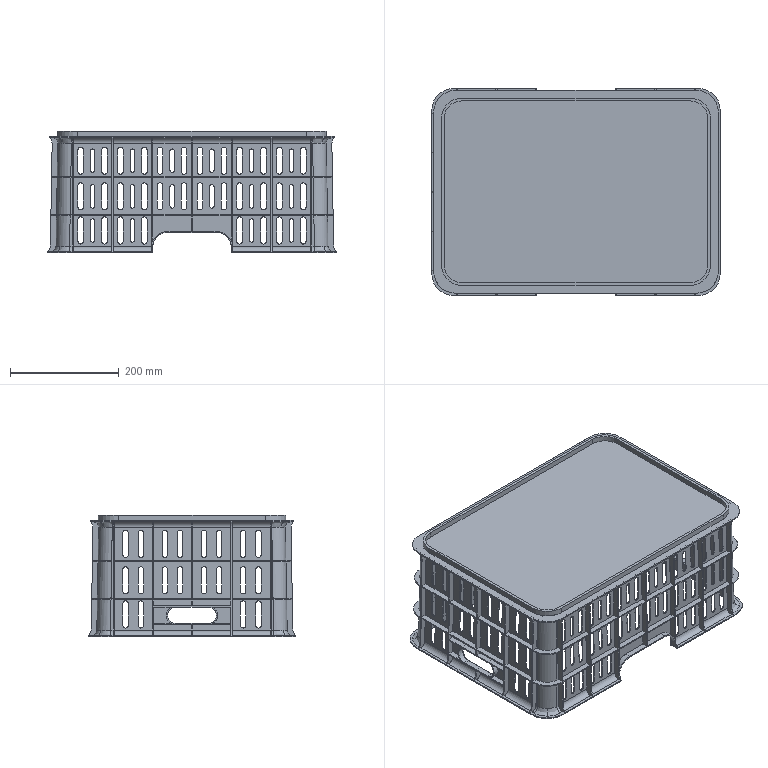Part | STEP file | SKRZYNIA_OWOCE1V11 | 1 solid | 1388 faces | box 530 x 380 x 224 mm | volume 1306449 mm3 | plane 742 | cylinder 610 | spline 36 | commonest cylinder face diameters 10 x312 8 x96 20 x80 40 x46 4 x14 50 x12